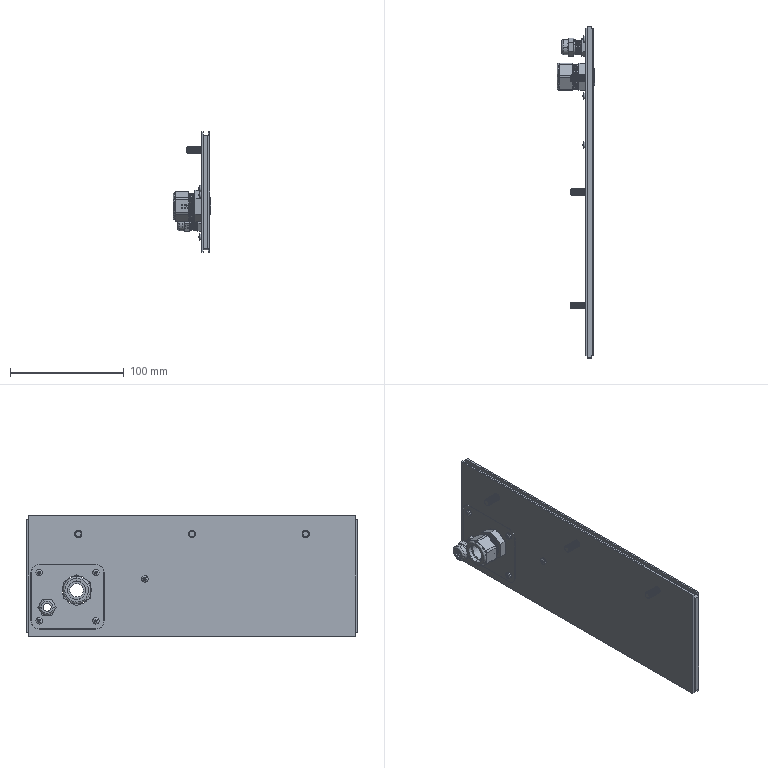Part | SolidWorks | 12 solids | 1593 faces | box 33.25 x 292 x 106 mm | volume 199269 mm3 | cone 698 | cylinder 604 | plane 261 | spline 16 | sphere 10 | torus 4 | commonest cylinder face diameters 3 x180 6 x160 11 x113 0.6 x25 21 x13 12.5 x11